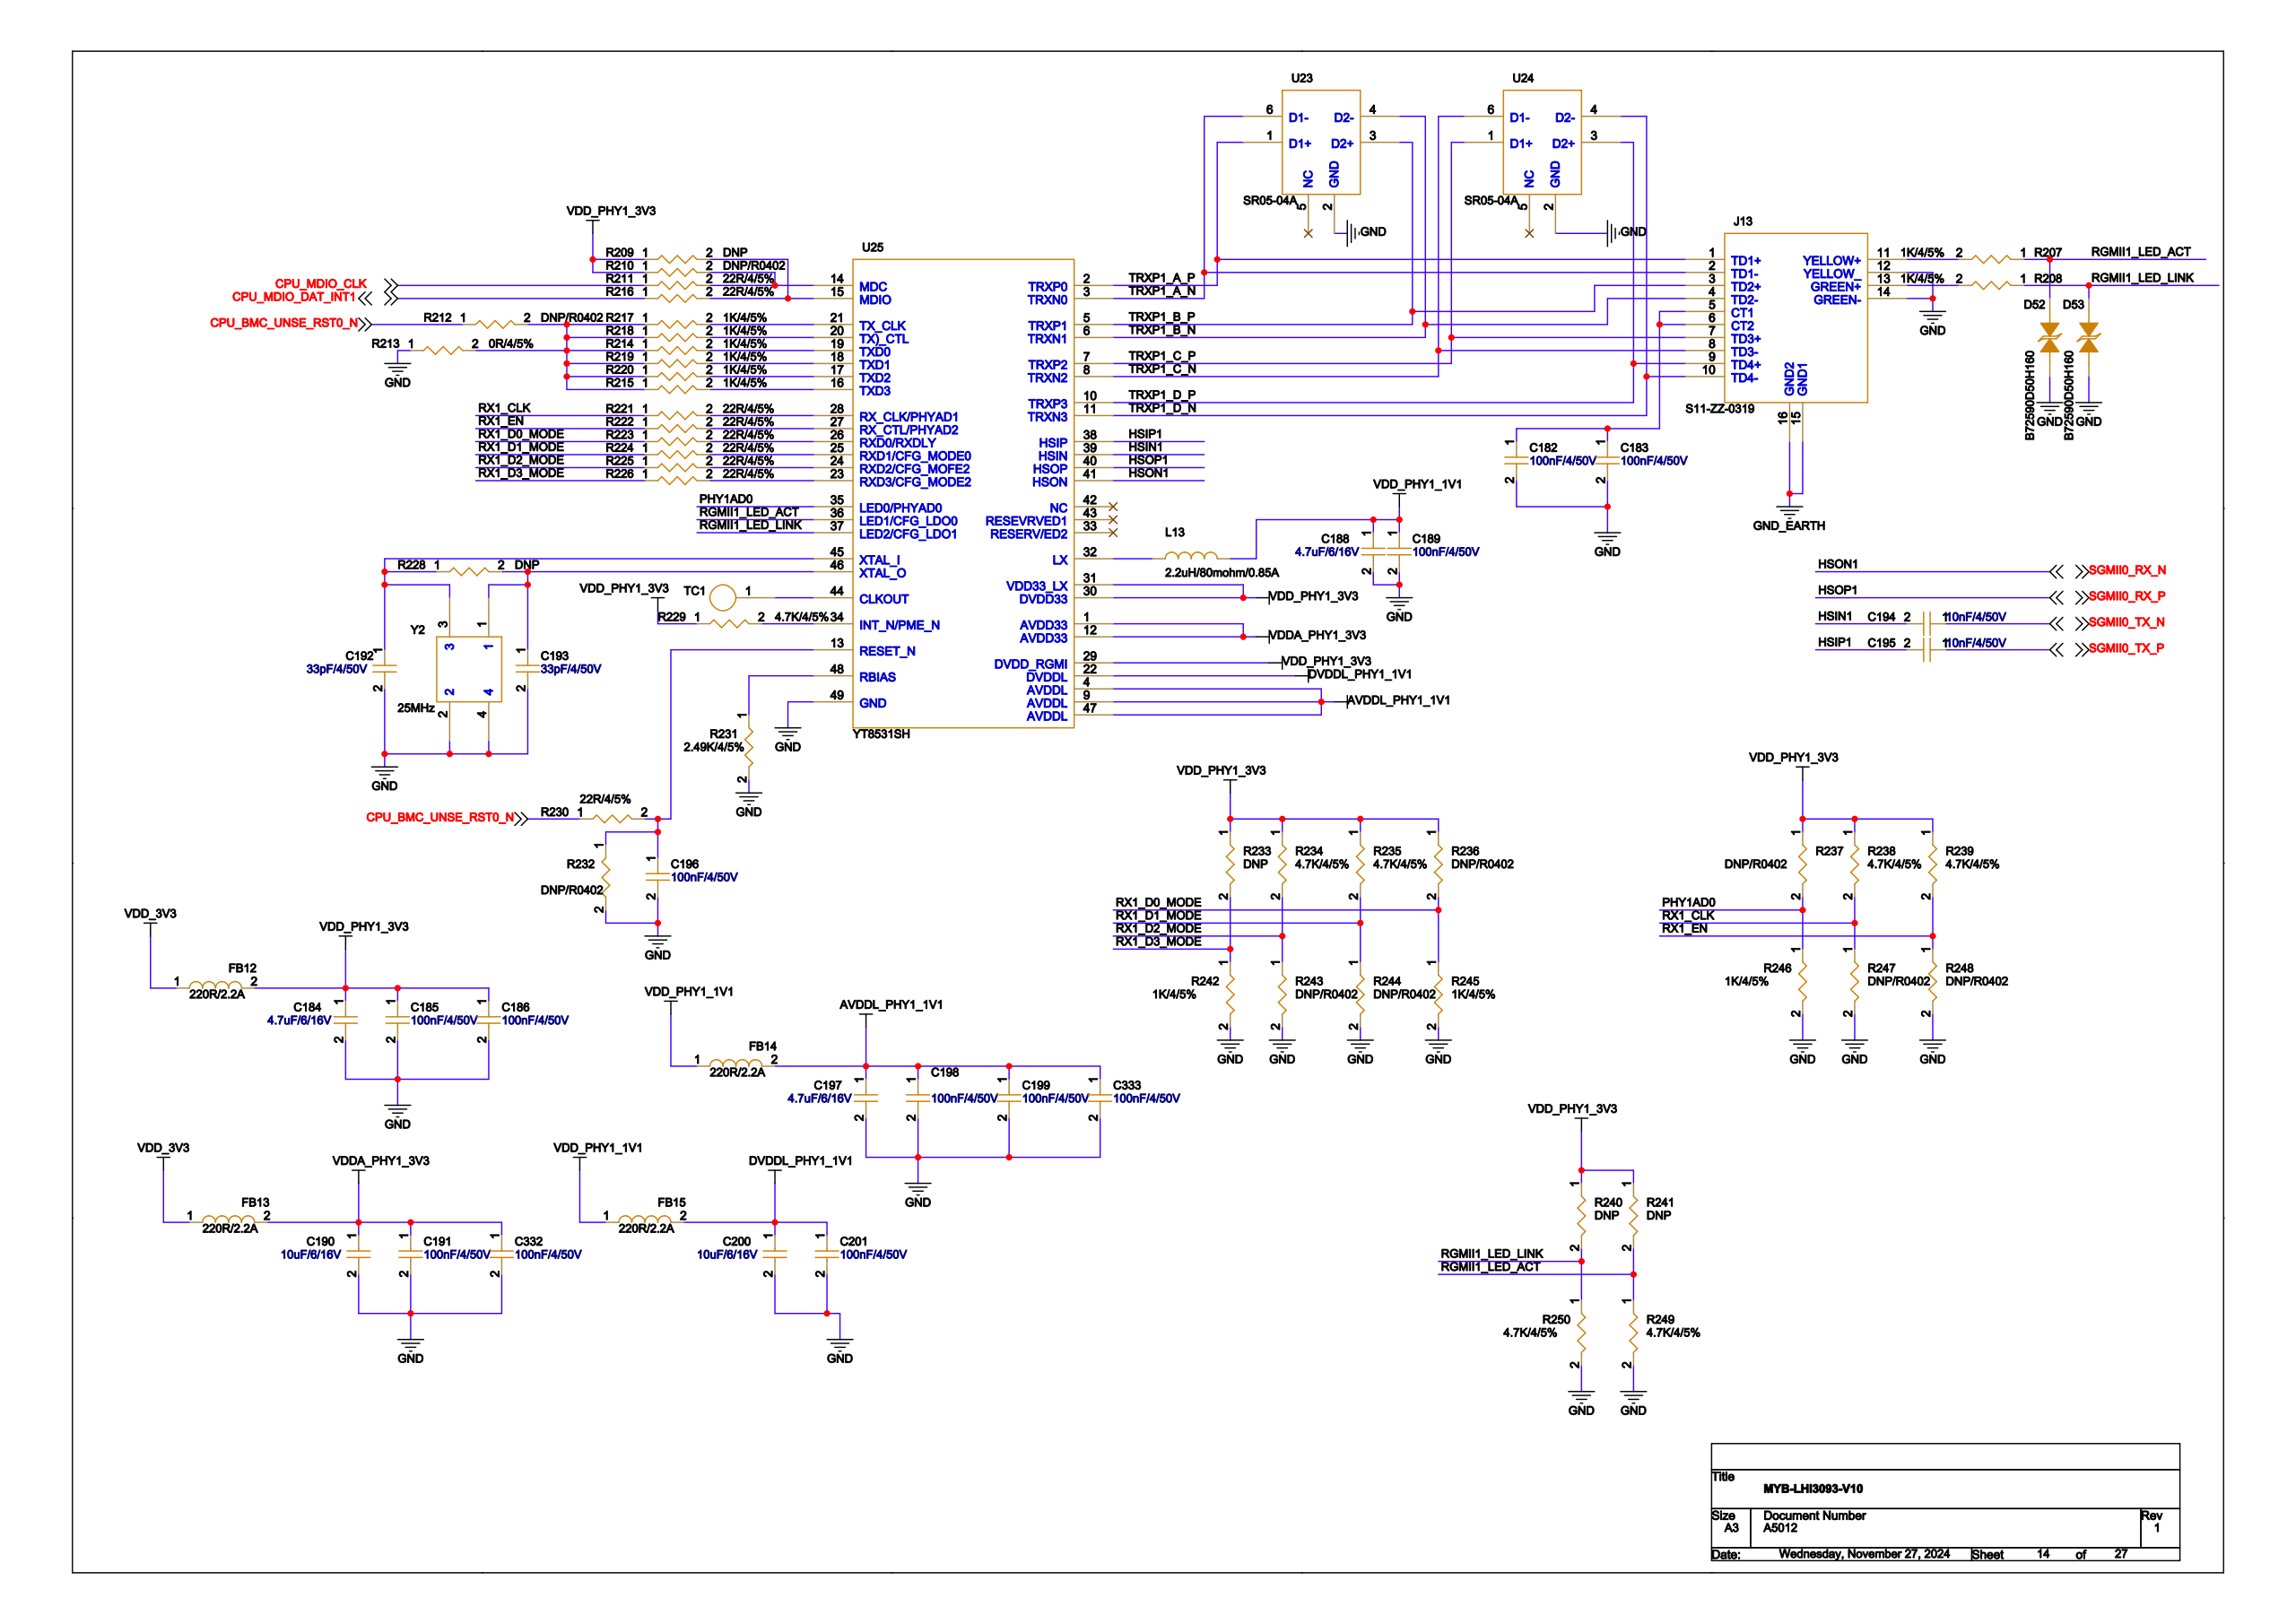Circuit board | Cadence Allegro | 1159 parts | 708 nets | one sheet of the schematic
Parts on this sheet (reference | value | footprint):
C182 | 100nF/4/50V | C0402
C183 | 100nF/4/50V | C0402
C184 | 4.7uF/6/16V | C0603
C185 | 100nF/4/50V | C0402
C186 | 100nF/4/50V | C0402
C188 | 4.7uF/6/16V | C0603
C189 | 100nF/4/50V | C0402
C190 | 10uF/6/16V | C0603
C191 | 100nF/4/50V | C0402
C192 | 33pF/4/50V | C0402
C193 | 33pF/4/50V | C0402
C194 | 10nF/4/50V | C0402
C195 | 10nF/4/50V | C0402
C196 | 100nF/4/50V | C0402
C197 | 4.7uF/6/16V | C0603
C198 | 100nF/4/50V | C0402
C199 | 100nF/4/50V | C0402
C200 | 10uF/6/16V | C0603
C201 | 100nF/4/50V | C0402
C332 | 100nF/4/50V | C0402
C333 | 100nF/4/50V | C0402
FB12 | 220R/2.2A | FB0603
FB13 | 220R/2.2A | FB0603
FB14 | 220R/2.2A | FB0603
FB15 | 220R/2.2A | FB0603
J13 | S11-ZZ-0319 | S11-ZZ-0319
L13 | 2.2uH/80mohm/0.85A | L2X2_5
R207 | 1K/4/5% | R0402
R208 | 1K/4/5% | R0402
R209 | DNP | R0402
R210 | DNP/R0402 | R0402
R211 | 22R/4/5% | R0402
R212 | DNP/R0402 | R0402
R213 | 0R/4/5% | R0402
R214 | 1K/4/5% | R0402
R215 | 1K/4/5% | R0402
R216 | 22R/4/5% | R0402
R217 | 1K/4/5% | R0402
R218 | 1K/4/5% | R0402
R219 | 1K/4/5% | R0402
R220 | 1K/4/5% | R0402
R221 | 22R/4/5% | R0402
R222 | 22R/4/5% | R0402
R223 | 22R/4/5% | R0402
R224 | 22R/4/5% | R0402
R225 | 22R/4/5% | R0402
R226 | 22R/4/5% | R0402
R228 | DNP | R0402
R229 | 4.7K/4/5% | R0402
R230 | 22R/4/5% | R0402
R231 | 2.49K/4/5% | R0402
R232 | DNP/R0402 | R0402
R233 | DNP | R0402
R234 | 4.7K/4/5% | R0402
R235 | 4.7K/4/5% | R0402
R236 | DNP/R0402 | R0402
R237 | DNP/R0402 | R0402
R238 | 4.7K/4/5% | R0402
R239 | 4.7K/4/5% | R0402
R240 | DNP | R0402
R241 | DNP | R0402
R242 | 1K/4/5% | R0402
R243 | DNP/R0402 | R0402
R244 | DNP/R0402 | R0402
R245 | 1K/4/5% | R0402
R246 | 1K/4/5% | R0402
R247 | DNP/R0402 | R0402
R248 | DNP/R0402 | R0402
R249 | 4.7K/4/5% | R0402
R250 | 4.7K/4/5% | R0402
TC1 | TP | TP_SMT
U23 | SR05-04A | SOT23-6
U24 | SR05-04A | SOT23-6
U25 | YT8531SH | QFN48-0_4
Y2 | 25MHz | 3225
Nets of these parts (net: part-pin ...):
GND: C182-2 C183-2 C184-2 C185-2 C186-2 C188-2 C189-2 C190-2 C191-2 C192-2 C193-2 C196-2 C197-2 C198-2 C199-2 C200-2 C201-2 C332-2 C333-2 J13-12 J13-14 R213-1 R231-2 R232-2 R242-2 R243-2 R244-2 R245-2 R246-2 R247-2 R248-2 R249-2 R250-2 U23-2 U24-2 Y2-2 Y2-4 U25-49
VDD_3V3: FB12-1 FB13-1
N14974064: C182-1 C183-1 J13-5 J13-6
VDD_PHY1_3V3: C184-1 C185-1 C186-1 FB12-2 R209-1 R210-1 R229-1 R233-1 R234-1 R235-1 R236-1 R237-1 R238-1 R239-1 R240-1 R241-1 U25-29 U25-30 U25-31
VDD_PHY1_1V1: C188-1 C189-1 FB14-1 FB15-1 L13-2
VDDA_PHY1_3V3: C190-1 C191-1 C332-1 FB13-2 U25-1 U25-12
N14970793: C196-1 R230-2 R232-1 U25-13
AVDDL_PHY1_1V1: C197-1 C198-1 C199-1 C333-1 FB14-2 U25-4 U25-9 U25-47
DVDDL_PHY1_1V1: C200-1 C201-1 FB15-2 U25-22
GND_EARTH: J13-15 J13-16
N14970304: C192-1 R228-1 Y2-3 U25-45
N14970203: C193-1 R228-2 Y2-1 U25-46
SGMII0_TX_N: C194-1
HSIN1: C194-2 U25-39
SGMII0_TX_P: C195-1
HSIP1: C195-2 U25-38
RGMII1_LED_ACT: R207-1 R241-2 R249-1 U25-36
RGMII1_LED_LINK: R208-1 R240-2 R250-1 U25-37
N14974927: J13-13 R208-2
TRXP1_A_P: J13-1 U23-1 U25-2
TRXP1_A_N: J13-2 U23-6 U25-3
TRXP1_B_P: J13-3 U23-3 U25-5
TRXP1_B_N: J13-4 U23-4 U25-6
TRXP1_C_P: J13-7 U24-1 U25-7
TRXP1_C_N: J13-8 U24-6 U25-8
TRXP1_D_P: J13-9 U24-3 U25-10
TRXP1_D_N: J13-10 U24-4 U25-11
N14974923: J13-11 R207-2
N14969764: R212-2 R213-2 R214-1 R215-1 R217-1 R218-1 R219-1 R220-1
N14969576: R214-2 U25-19
N14969588: R215-2 U25-16
N14969568: R217-2 U25-21
N14969572: R218-2 U25-20
N14969580: R219-2 U25-18
N14969584: R220-2 U25-17
RX1_D3_MODE: R226-1 R233-2 R242-1
RX1_D0_MODE: R223-1 R236-2 R245-1
PHY1AD0: R237-2 R246-1 U25-35
CPU_MDIO_CLK: R211-1
N14969510: R210-2 R211-2 U25-14
CPU_MDIO_DAT_INT1: R216-1
N14969514: R209-2 R216-2 U25-15
RX1_CLK: R221-1 R238-2 R247-1
N14969592: R221-2 U25-28
RX1_EN: R222-1 R239-2 R248-1
N14969596: R222-2 U25-27
N14969600: R223-2 U25-26
RX1_D1_MODE: R224-1 R235-2 R244-1
N14969604: R224-2 U25-25
RX1_D2_MODE: R225-1 R234-2 R243-1
N14969608: R225-2 U25-24
N14969612: R226-2 U25-23
CPU_BMC_UNSE_RST0_N: R212-1 R230-1
N14970615: R229-2 U25-34
N14970702: R231-1 U25-48
N14970572: TC1-1 U25-44
SGMII0_RX_N: U25-41
SGMII0_RX_P: U25-40
N14972923: L13-1 U25-32